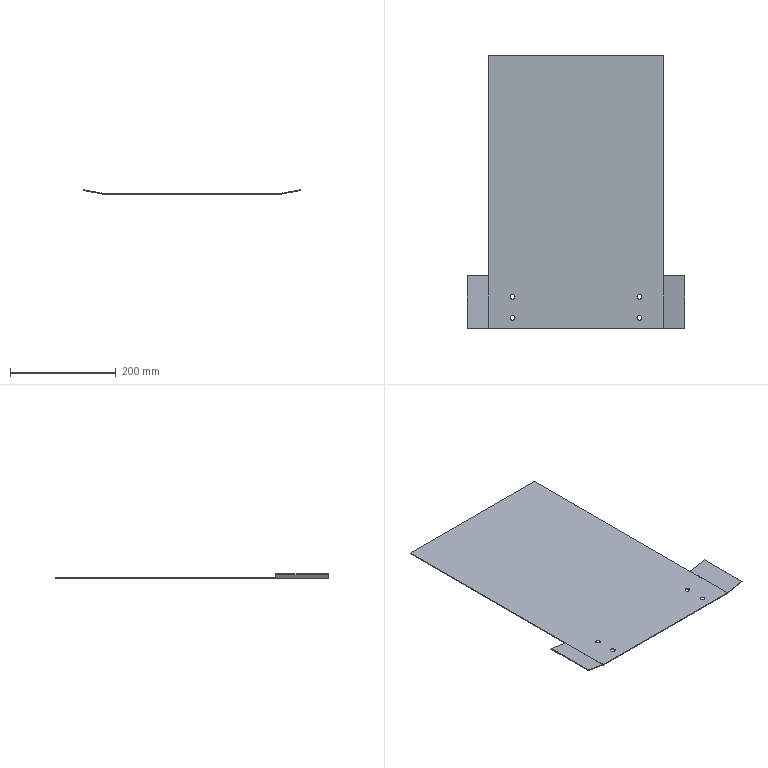Part | SolidWorks | features EdgeFlange 1, FlatPattern 1, ICE 1, SMBaseFlange 1, SheetMetal 1 | 1 solid | 32 faces | box 411.771 x 517 x 8.423 mm | volume 269565 mm3 | plane 20 | cylinder 12 | commonest cylinder face diameters 9 x8 1.473 x2 4.473 x2
STEP:
#1=CARTESIAN_POINT('',(-124.5,-30.,-1.5));
#2=VERTEX_POINT('',#1);
#3=CARTESIAN_POINT('',(-115.5,-30.,-1.5));
#4=VERTEX_POINT('',#3);
#5=CARTESIAN_POINT('',(-120.,-30.,-1.5));
#6=DIRECTION('',(0.,0.,1.));
#7=DIRECTION('',(1.,0.,0.));
#8=AXIS2_PLACEMENT_3D('',#5,#6,#7);
#9=CIRCLE('',#8,4.5);
#10=EDGE_CURVE('',#2,#4,#9,.T.);
#11=ORIENTED_EDGE('',*,*,#10,.F.);
#12=CARTESIAN_POINT('',(-124.5,-30.,0.));
#13=VERTEX_POINT('',#12);
#14=CARTESIAN_POINT('',(-124.5,-30.,-1.5));
#15=DIRECTION('',(0.,0.,1.));
#16=VECTOR('',#15,1000.);
#17=LINE('',#14,#16);
#18=EDGE_CURVE('',#2,#13,#17,.T.);
#19=ORIENTED_EDGE('',*,*,#18,.T.);
#20=CARTESIAN_POINT('',(-115.5,-30.,0.));
#21=VERTEX_POINT('',#20);
#22=CARTESIAN_POINT('',(-120.,-30.,0.));
#23=DIRECTION('',(0.,0.,1.));
#24=DIRECTION('',(1.,0.,0.));
#25=AXIS2_PLACEMENT_3D('',#22,#23,#24);
#26=CIRCLE('',#25,4.5);
#27=EDGE_CURVE('',#13,#21,#26,.T.);
#28=ORIENTED_EDGE('',*,*,#27,.T.);
#29=CARTESIAN_POINT('',(-115.5,-30.,-1.5));
#30=DIRECTION('',(0.,0.,1.));
#31=VECTOR('',#30,1000.);
#32=LINE('',#29,#31);
#33=EDGE_CURVE('',#4,#21,#32,.T.);
#34=ORIENTED_EDGE('',*,*,#33,.F.);
#35=EDGE_LOOP('',(#11,#19,#28,#34));
#36=FACE_OUTER_BOUND('',#35,.T.);
#37=CARTESIAN_POINT('',(-120.,-30.,-1.5));
#38=DIRECTION('',(0.,0.,1.));
#39=DIRECTION('',(1.,0.,0.));
#40=AXIS2_PLACEMENT_3D('',#37,#38,#39);
#41=CYLINDRICAL_SURFACE('',#40,4.5);
#42=ADVANCED_FACE('',(#36),#41,.F.);
#43=CARTESIAN_POINT('',(-124.5,10.,-1.5));
#44=VERTEX_POINT('',#43);
#45=CARTESIAN_POINT('',(-115.5,10.,-1.5));
#46=VERTEX_POINT('',#45);
#47=CARTESIAN_POINT('',(-120.,10.,-1.5));
#48=DIRECTION('',(0.,0.,1.));
#49=DIRECTION('',(1.,0.,0.));
#50=AXIS2_PLACEMENT_3D('',#47,#48,#49);
#51=CIRCLE('',#50,4.5);
#52=EDGE_CURVE('',#44,#46,#51,.T.);
#53=ORIENTED_EDGE('',*,*,#52,.F.);
#54=CARTESIAN_POINT('',(-124.5,10.,0.));
#55=VERTEX_POINT('',#54);
#56=CARTESIAN_POINT('',(-124.5,10.,-1.5));
#57=DIRECTION('',(0.,0.,1.));
#58=VECTOR('',#57,1000.);
#59=LINE('',#56,#58);
#60=EDGE_CURVE('',#44,#55,#59,.T.);
#61=ORIENTED_EDGE('',*,*,#60,.T.);
#62=CARTESIAN_POINT('',(-115.5,10.,0.));
#63=VERTEX_POINT('',#62);
#64=CARTESIAN_POINT('',(-120.,10.,0.));
#65=DIRECTION('',(0.,0.,1.));
#66=DIRECTION('',(1.,0.,0.));
#67=AXIS2_PLACEMENT_3D('',#64,#65,#66);
#68=CIRCLE('',#67,4.5);
#69=EDGE_CURVE('',#55,#63,#68,.T.);
#70=ORIENTED_EDGE('',*,*,#69,.T.);
#71=CARTESIAN_POINT('',(-115.5,10.,-1.5));
#72=DIRECTION('',(0.,0.,1.));
#73=VECTOR('',#72,1000.);
#74=LINE('',#71,#73);
#75=EDGE_CURVE('',#46,#63,#74,.T.);
#76=ORIENTED_EDGE('',*,*,#75,.F.);
#77=EDGE_LOOP('',(#53,#61,#70,#76));
#78=FACE_OUTER_BOUND('',#77,.T.);
#79=CARTESIAN_POINT('',(-120.,10.,-1.5));
#80=DIRECTION('',(0.,0.,1.));
#81=DIRECTION('',(1.,0.,0.));
#82=AXIS2_PLACEMENT_3D('',#79,#80,#81);
#83=CYLINDRICAL_SURFACE('',#82,4.5);
#84=ADVANCED_FACE('',(#78),#83,.F.);
#85=CARTESIAN_POINT('',(115.5,-30.,-1.5));
#86=VERTEX_POINT('',#85);
#87=CARTESIAN_POINT('',(124.5,-30.,-1.5));
#88=VERTEX_POINT('',#87);
#89=CARTESIAN_POINT('',(120.,-30.,-1.5));
#90=DIRECTION('',(0.,0.,1.));
#91=DIRECTION('',(1.,0.,0.));
#92=AXIS2_PLACEMENT_3D('',#89,#90,#91);
#93=CIRCLE('',#92,4.5);
#94=EDGE_CURVE('',#86,#88,#93,.T.);
#95=ORIENTED_EDGE('',*,*,#94,.F.);
#96=CARTESIAN_POINT('',(115.5,-30.,0.));
#97=VERTEX_POINT('',#96);
#98=CARTESIAN_POINT('',(115.5,-30.,-1.5));
#99=DIRECTION('',(0.,0.,1.));
#100=VECTOR('',#99,1000.);
#101=LINE('',#98,#100);
#102=EDGE_CURVE('',#86,#97,#101,.T.);
#103=ORIENTED_EDGE('',*,*,#102,.T.);
#104=CARTESIAN_POINT('',(124.5,-30.,0.));
#105=VERTEX_POINT('',#104);
#106=CARTESIAN_POINT('',(120.,-30.,0.));
#107=DIRECTION('',(0.,0.,1.));
#108=DIRECTION('',(1.,0.,0.));
#109=AXIS2_PLACEMENT_3D('',#106,#107,#108);
#110=CIRCLE('',#109,4.5);
#111=EDGE_CURVE('',#97,#105,#110,.T.);
#112=ORIENTED_EDGE('',*,*,#111,.T.);
#113=CARTESIAN_POINT('',(124.5,-30.,-1.5));
#114=DIRECTION('',(0.,0.,1.));
#115=VECTOR('',#114,1000.);
#116=LINE('',#113,#115);
#117=EDGE_CURVE('',#88,#105,#116,.T.);
#118=ORIENTED_EDGE('',*,*,#117,.F.);
#119=EDGE_LOOP('',(#95,#103,#112,#118));
#120=FACE_OUTER_BOUND('',#119,.T.);
#121=CARTESIAN_POINT('',(120.,-30.,-1.5));
#122=DIRECTION('',(0.,0.,1.));
#123=DIRECTION('',(1.,0.,0.));
#124=AXIS2_PLACEMENT_3D('',#121,#122,#123);
#125=CYLINDRICAL_SURFACE('',#124,4.5);
#126=ADVANCED_FACE('',(#120),#125,.F.);
#127=CARTESIAN_POINT('',(115.5,10.,-1.5));
#128=VERTEX_POINT('',#127);
#129=CARTESIAN_POINT('',(124.5,10.,-1.5));
#130=VERTEX_POINT('',#129);
#131=CARTESIAN_POINT('',(120.,10.,-1.5));
#132=DIRECTION('',(0.,0.,1.));
#133=DIRECTION('',(1.,0.,0.));
#134=AXIS2_PLACEMENT_3D('',#131,#132,#133);
#135=CIRCLE('',#134,4.5);
#136=EDGE_CURVE('',#128,#130,#135,.T.);
#137=ORIENTED_EDGE('',*,*,#136,.F.);
#138=CARTESIAN_POINT('',(115.5,10.,0.));
#139=VERTEX_POINT('',#138);
#140=CARTESIAN_POINT('',(115.5,10.,-1.5));
#141=DIRECTION('',(0.,0.,1.));
#142=VECTOR('',#141,1000.);
#143=LINE('',#140,#142);
#144=EDGE_CURVE('',#128,#139,#143,.T.);
#145=ORIENTED_EDGE('',*,*,#144,.T.);
#146=CARTESIAN_POINT('',(124.5,10.,0.));
#147=VERTEX_POINT('',#146);
#148=CARTESIAN_POINT('',(120.,10.,0.));
#149=DIRECTION('',(0.,0.,1.));
#150=DIRECTION('',(1.,0.,0.));
#151=AXIS2_PLACEMENT_3D('',#148,#149,#150);
#152=CIRCLE('',#151,4.5);
#153=EDGE_CURVE('',#139,#147,#152,.T.);
#154=ORIENTED_EDGE('',*,*,#153,.T.);
#155=CARTESIAN_POINT('',(124.5,10.,-1.5));
#156=DIRECTION('',(0.,0.,1.));
#157=VECTOR('',#156,1000.);
#158=LINE('',#155,#157);
#159=EDGE_CURVE('',#130,#147,#158,.T.);
#160=ORIENTED_EDGE('',*,*,#159,.F.);
#161=EDGE_LOOP('',(#137,#145,#154,#160));
#162=FACE_OUTER_BOUND('',#161,.T.);
#163=CARTESIAN_POINT('',(120.,10.,-1.5));
#164=DIRECTION('',(0.,0.,1.));
#165=DIRECTION('',(1.,0.,0.));
#166=AXIS2_PLACEMENT_3D('',#163,#164,#165);
#167=CYLINDRICAL_SURFACE('',#166,4.5);
#168=ADVANCED_FACE('',(#162),#167,.F.);
#169=CARTESIAN_POINT('',(-120.,-30.,-1.5));
#170=DIRECTION('',(0.,0.,1.));
#171=DIRECTION('',(1.,0.,0.));
#172=AXIS2_PLACEMENT_3D('',#169,#170,#171);
#173=CIRCLE('',#172,4.5);
#174=EDGE_CURVE('',#4,#2,#173,.T.);
#175=ORIENTED_EDGE('',*,*,#174,.T.);
#176=ORIENTED_EDGE('',*,*,#10,.T.);
#177=EDGE_LOOP('',(#175,#176));
#178=FACE_BOUND('',#177,.T.);
#179=CARTESIAN_POINT('',(-120.,10.,-1.5));
#180=DIRECTION('',(0.,0.,1.));
#181=DIRECTION('',(1.,0.,0.));
#182=AXIS2_PLACEMENT_3D('',#179,#180,#181);
#183=CIRCLE('',#182,4.5);
#184=EDGE_CURVE('',#46,#44,#183,.T.);
#185=ORIENTED_EDGE('',*,*,#184,.T.);
#186=ORIENTED_EDGE('',*,*,#52,.T.);
#187=EDGE_LOOP('',(#185,#186));
#188=FACE_BOUND('',#187,.T.);
#189=CARTESIAN_POINT('',(120.,-30.,-1.5));
#190=DIRECTION('',(0.,0.,1.));
#191=DIRECTION('',(1.,0.,0.));
#192=AXIS2_PLACEMENT_3D('',#189,#190,#191);
#193=CIRCLE('',#192,4.5);
#194=EDGE_CURVE('',#88,#86,#193,.T.);
#195=ORIENTED_EDGE('',*,*,#194,.T.);
#196=ORIENTED_EDGE('',*,*,#94,.T.);
#197=EDGE_LOOP('',(#195,#196));
#198=FACE_BOUND('',#197,.T.);
#199=CARTESIAN_POINT('',(120.,10.,-1.5));
#200=DIRECTION('',(0.,0.,1.));
#201=DIRECTION('',(1.,0.,0.));
#202=AXIS2_PLACEMENT_3D('',#199,#200,#201);
#203=CIRCLE('',#202,4.5);
#204=EDGE_CURVE('',#130,#128,#203,.T.);
#205=ORIENTED_EDGE('',*,*,#204,.T.);
#206=ORIENTED_EDGE('',*,*,#136,.T.);
#207=EDGE_LOOP('',(#205,#206));
#208=FACE_BOUND('',#207,.T.);
#209=CARTESIAN_POINT('',(-166.297,-50.,-1.5));
#210=VERTEX_POINT('',#209);
#211=CARTESIAN_POINT('',(-166.297,50.,-1.5));
#212=VERTEX_POINT('',#211);
#213=CARTESIAN_POINT('',(-166.297,-50.,-1.5));
#214=DIRECTION('',(0.,1.,0.));
#215=VECTOR('',#214,1000.);
#216=LINE('',#213,#215);
#217=EDGE_CURVE('',#210,#212,#216,.T.);
#218=ORIENTED_EDGE('',*,*,#217,.T.);
#219=CARTESIAN_POINT('',(-166.297,467.,-1.5));
#220=VERTEX_POINT('',#219);
#221=CARTESIAN_POINT('',(-166.297,467.,-1.5));
#222=DIRECTION('',(0.,-1.,0.));
#223=VECTOR('',#222,1000.);
#224=LINE('',#221,#223);
#225=EDGE_CURVE('',#220,#212,#224,.T.);
#226=ORIENTED_EDGE('',*,*,#225,.F.);
#227=CARTESIAN_POINT('',(166.297,467.,-1.5));
#228=VERTEX_POINT('',#227);
#229=CARTESIAN_POINT('',(166.297,467.,-1.5));
#230=DIRECTION('',(-1.,0.,0.));
#231=VECTOR('',#230,1000.);
#232=LINE('',#229,#231);
#233=EDGE_CURVE('',#228,#220,#232,.T.);
#234=ORIENTED_EDGE('',*,*,#233,.F.);
#235=CARTESIAN_POINT('',(166.297,50.,-1.5));
#236=VERTEX_POINT('',#235);
#237=CARTESIAN_POINT('',(166.297,467.,-1.5));
#238=DIRECTION('',(0.,-1.,0.));
#239=VECTOR('',#238,1000.);
#240=LINE('',#237,#239);
#241=EDGE_CURVE('',#228,#236,#240,.T.);
#242=ORIENTED_EDGE('',*,*,#241,.T.);
#243=CARTESIAN_POINT('',(166.297,-50.,-1.5));
#244=VERTEX_POINT('',#243);
#245=CARTESIAN_POINT('',(166.297,50.,-1.5));
#246=DIRECTION('',(0.,-1.,0.));
#247=VECTOR('',#246,1000.);
#248=LINE('',#245,#247);
#249=EDGE_CURVE('',#236,#244,#248,.T.);
#250=ORIENTED_EDGE('',*,*,#249,.T.);
#251=CARTESIAN_POINT('',(-175.,-50.,-1.5));
#252=DIRECTION('',(1.,0.,0.));
#253=VECTOR('',#252,1000.);
#254=LINE('',#251,#253);
#255=EDGE_CURVE('',#210,#244,#254,.T.);
#256=ORIENTED_EDGE('',*,*,#255,.F.);
#257=EDGE_LOOP('',(#218,#226,#234,#242,#250,#256));
#258=FACE_OUTER_BOUND('',#257,.T.);
#259=CARTESIAN_POINT('',(0.,0.,-1.5));
#260=DIRECTION('',(0.,0.,-1.));
#261=DIRECTION('',(-1.,0.,0.));
#262=AXIS2_PLACEMENT_3D('',#259,#260,#261);
#263=PLANE('',#262);
#264=ADVANCED_FACE('',(#178,#188,#198,#208,#258),#263,.T.);
#265=CARTESIAN_POINT('',(-120.,-30.,0.));
#266=DIRECTION('',(0.,0.,1.));
#267=DIRECTION('',(1.,0.,0.));
#268=AXIS2_PLACEMENT_3D('',#265,#266,#267);
#269=CIRCLE('',#268,4.5);
#270=EDGE_CURVE('',#21,#13,#269,.T.);
#271=ORIENTED_EDGE('',*,*,#270,.F.);
#272=ORIENTED_EDGE('',*,*,#27,.F.);
#273=EDGE_LOOP('',(#271,#272));
#274=FACE_BOUND('',#273,.T.);
#275=CARTESIAN_POINT('',(-120.,10.,0.));
#276=DIRECTION('',(0.,0.,1.));
#277=DIRECTION('',(1.,0.,0.));
#278=AXIS2_PLACEMENT_3D('',#275,#276,#277);
#279=CIRCLE('',#278,4.5);
#280=EDGE_CURVE('',#63,#55,#279,.T.);
#281=ORIENTED_EDGE('',*,*,#280,.F.);
#282=ORIENTED_EDGE('',*,*,#69,.F.);
#283=EDGE_LOOP('',(#281,#282));
#284=FACE_BOUND('',#283,.T.);
#285=CARTESIAN_POINT('',(120.,-30.,0.));
#286=DIRECTION('',(0.,0.,1.));
#287=DIRECTION('',(1.,0.,0.));
#288=AXIS2_PLACEMENT_3D('',#285,#286,#287);
#289=CIRCLE('',#288,4.5);
#290=EDGE_CURVE('',#105,#97,#289,.T.);
#291=ORIENTED_EDGE('',*,*,#290,.F.);
#292=ORIENTED_EDGE('',*,*,#111,.F.);
#293=EDGE_LOOP('',(#291,#292));
#294=FACE_BOUND('',#293,.T.);
#295=CARTESIAN_POINT('',(120.,10.,0.));
#296=DIRECTION('',(0.,0.,1.));
#297=DIRECTION('',(1.,0.,0.));
#298=AXIS2_PLACEMENT_3D('',#295,#296,#297);
#299=CIRCLE('',#298,4.5);
#300=EDGE_CURVE('',#147,#139,#299,.T.);
#301=ORIENTED_EDGE('',*,*,#300,.F.);
#302=ORIENTED_EDGE('',*,*,#153,.F.);
#303=EDGE_LOOP('',(#301,#302));
#304=FACE_BOUND('',#303,.T.);
#305=CARTESIAN_POINT('',(166.297,50.,0.));
#306=VERTEX_POINT('',#305);
#307=CARTESIAN_POINT('',(166.297,-50.,0.));
#308=VERTEX_POINT('',#307);
#309=CARTESIAN_POINT('',(166.297,50.,0.));
#310=DIRECTION('',(0.,-1.,0.));
#311=VECTOR('',#310,1000.);
#312=LINE('',#309,#311);
#313=EDGE_CURVE('',#306,#308,#312,.T.);
#314=ORIENTED_EDGE('',*,*,#313,.F.);
#315=CARTESIAN_POINT('',(166.297,467.,0.));
#316=VERTEX_POINT('',#315);
#317=CARTESIAN_POINT('',(166.297,467.,0.));
#318=DIRECTION('',(0.,-1.,0.));
#319=VECTOR('',#318,1000.);
#320=LINE('',#317,#319);
#321=EDGE_CURVE('',#316,#306,#320,.T.);
#322=ORIENTED_EDGE('',*,*,#321,.F.);
#323=CARTESIAN_POINT('',(-166.297,467.,0.));
#324=VERTEX_POINT('',#323);
#325=CARTESIAN_POINT('',(-166.297,467.,0.));
#326=DIRECTION('',(1.,0.,0.));
#327=VECTOR('',#326,1000.);
#328=LINE('',#325,#327);
#329=EDGE_CURVE('',#324,#316,#328,.T.);
#330=ORIENTED_EDGE('',*,*,#329,.F.);
#331=CARTESIAN_POINT('',(-166.297,50.,0.));
#332=VERTEX_POINT('',#331);
#333=CARTESIAN_POINT('',(-166.297,467.,0.));
#334=DIRECTION('',(0.,-1.,0.));
#335=VECTOR('',#334,1000.);
#336=LINE('',#333,#335);
#337=EDGE_CURVE('',#324,#332,#336,.T.);
#338=ORIENTED_EDGE('',*,*,#337,.T.);
#339=CARTESIAN_POINT('',(-166.297,-50.,0.));
#340=VERTEX_POINT('',#339);
#341=CARTESIAN_POINT('',(-166.297,-50.,0.));
#342=DIRECTION('',(0.,1.,0.));
#343=VECTOR('',#342,1000.);
#344=LINE('',#341,#343);
#345=EDGE_CURVE('',#340,#332,#344,.T.);
#346=ORIENTED_EDGE('',*,*,#345,.F.);
#347=CARTESIAN_POINT('',(-175.,-50.,0.));
#348=DIRECTION('',(1.,0.,0.));
#349=VECTOR('',#348,1000.);
#350=LINE('',#347,#349);
#351=EDGE_CURVE('',#340,#308,#350,.T.);
#352=ORIENTED_EDGE('',*,*,#351,.T.);
#353=EDGE_LOOP('',(#314,#322,#330,#338,#346,#352));
#354=FACE_OUTER_BOUND('',#353,.T.);
#355=CARTESIAN_POINT('',(0.,0.,0.));
#356=DIRECTION('',(0.,0.,-1.));
#357=DIRECTION('',(-1.,0.,0.));
#358=AXIS2_PLACEMENT_3D('',#355,#356,#357);
#359=PLANE('',#358);
#360=ADVANCED_FACE('',(#274,#284,#294,#304,#354),#359,.F.);
#361=CARTESIAN_POINT('',(166.297,-50.,0.));
#362=DIRECTION('',(0.,0.,-1.));
#363=VECTOR('',#362,1000.);
#364=LINE('',#361,#363);
#365=EDGE_CURVE('',#308,#244,#364,.T.);
#366=ORIENTED_EDGE('',*,*,#365,.F.);
#367=ORIENTED_EDGE('',*,*,#351,.F.);
#368=CARTESIAN_POINT('',(-166.297,-50.,0.));
#369=DIRECTION('',(0.,0.,-1.));
#370=VECTOR('',#369,1000.);
#371=LINE('',#368,#370);
#372=EDGE_CURVE('',#340,#210,#371,.T.);
#373=ORIENTED_EDGE('',*,*,#372,.T.);
#374=ORIENTED_EDGE('',*,*,#255,.T.);
#375=EDGE_LOOP('',(#366,#367,#373,#374));
#376=FACE_OUTER_BOUND('',#375,.T.);
#377=CARTESIAN_POINT('',(-175.,-50.,-1.5));
#378=DIRECTION('',(0.,-1.,0.));
#379=DIRECTION('',(0.,0.,-1.));
#380=AXIS2_PLACEMENT_3D('',#377,#378,#379);
#381=PLANE('',#380);
#382=ADVANCED_FACE('',(#376),#381,.T.);
#383=ORIENTED_EDGE('',*,*,#144,.F.);
#384=ORIENTED_EDGE('',*,*,#204,.F.);
#385=ORIENTED_EDGE('',*,*,#159,.T.);
#386=ORIENTED_EDGE('',*,*,#300,.T.);
#387=EDGE_LOOP('',(#383,#384,#385,#386));
#388=FACE_OUTER_BOUND('',#387,.T.);
#389=CARTESIAN_POINT('',(120.,10.,-1.5));
#390=DIRECTION('',(0.,0.,1.));
#391=DIRECTION('',(1.,0.,0.));
#392=AXIS2_PLACEMENT_3D('',#389,#390,#391);
#393=CYLINDRICAL_SURFACE('',#392,4.5);
#394=ADVANCED_FACE('',(#388),#393,.F.);
#395=ORIENTED_EDGE('',*,*,#102,.F.);
#396=ORIENTED_EDGE('',*,*,#194,.F.);
#397=ORIENTED_EDGE('',*,*,#117,.T.);
#398=ORIENTED_EDGE('',*,*,#290,.T.);
#399=EDGE_LOOP('',(#395,#396,#397,#398));
#400=FACE_OUTER_BOUND('',#399,.T.);
#401=CARTESIAN_POINT('',(120.,-30.,-1.5));
#402=DIRECTION('',(0.,0.,1.));
#403=DIRECTION('',(1.,0.,0.));
#404=AXIS2_PLACEMENT_3D('',#401,#402,#403);
#405=CYLINDRICAL_SURFACE('',#404,4.5);
#406=ADVANCED_FACE('',(#400),#405,.F.);
#407=ORIENTED_EDGE('',*,*,#60,.F.);
#408=ORIENTED_EDGE('',*,*,#184,.F.);
#409=ORIENTED_EDGE('',*,*,#75,.T.);
#410=ORIENTED_EDGE('',*,*,#280,.T.);
#411=EDGE_LOOP('',(#407,#408,#409,#410));
#412=FACE_OUTER_BOUND('',#411,.T.);
#413=CARTESIAN_POINT('',(-120.,10.,-1.5));
#414=DIRECTION('',(0.,0.,1.));
#415=DIRECTION('',(1.,0.,0.));
#416=AXIS2_PLACEMENT_3D('',#413,#414,#415);
#417=CYLINDRICAL_SURFACE('',#416,4.5);
#418=ADVANCED_FACE('',(#412),#417,.F.);
#419=ORIENTED_EDGE('',*,*,#18,.F.);
#420=ORIENTED_EDGE('',*,*,#174,.F.);
#421=ORIENTED_EDGE('',*,*,#33,.T.);
#422=ORIENTED_EDGE('',*,*,#270,.T.);
#423=EDGE_LOOP('',(#419,#420,#421,#422));
#424=FACE_OUTER_BOUND('',#423,.T.);
#425=CARTESIAN_POINT('',(-120.,-30.,-1.5));
#426=DIRECTION('',(0.,0.,1.));
#427=DIRECTION('',(1.,0.,0.));
#428=AXIS2_PLACEMENT_3D('',#425,#426,#427);
#429=CYLINDRICAL_SURFACE('',#428,4.5);
#430=ADVANCED_FACE('',(#424),#429,.F.);
#431=CARTESIAN_POINT('',(-166.425,50.,0.01119));
#432=VERTEX_POINT('',#431);
#433=CARTESIAN_POINT('',(-166.686,50.,-1.466));
#434=VERTEX_POINT('',#433);
#435=CARTESIAN_POINT('',(-166.686,50.,-1.466));
#436=DIRECTION('',(-0.1736,0.,-0.9848));
#437=VECTOR('',#436,1000.);
#438=LINE('',#435,#437);
#439=EDGE_CURVE('',#432,#434,#438,.T.);
#440=ORIENTED_EDGE('',*,*,#439,.F.);
#441=CARTESIAN_POINT('',(-166.297,50.,0.7366));
#442=DIRECTION('',(0.,1.,0.));
#443=DIRECTION('',(0.,0.,-1.));
#444=AXIS2_PLACEMENT_3D('',#441,#442,#443);
#445=CIRCLE('',#444,0.7366);
#446=EDGE_CURVE('',#332,#432,#445,.T.);
#447=ORIENTED_EDGE('',*,*,#446,.F.);
#448=CARTESIAN_POINT('',(-166.297,50.,0.));
#449=DIRECTION('',(0.,0.,-1.));
#450=VECTOR('',#449,1000.);
#451=LINE('',#448,#450);
#452=EDGE_CURVE('',#332,#212,#451,.T.);
#453=ORIENTED_EDGE('',*,*,#452,.T.);
#454=CARTESIAN_POINT('',(-166.297,50.,0.7366));
#455=DIRECTION('',(0.,1.,0.));
#456=DIRECTION('',(0.,0.,-1.));
#457=AXIS2_PLACEMENT_3D('',#454,#455,#456);
#458=CIRCLE('',#457,2.237);
#459=EDGE_CURVE('',#212,#434,#458,.T.);
#460=ORIENTED_EDGE('',*,*,#459,.T.);
#461=EDGE_LOOP('',(#440,#447,#453,#460));
#462=FACE_OUTER_BOUND('',#461,.T.);
#463=CARTESIAN_POINT('',(-166.297,50.,0.7366));
#464=DIRECTION('',(0.,1.,0.));
#465=DIRECTION('',(0.,0.,1.));
#466=AXIS2_PLACEMENT_3D('',#463,#464,#465);
#467=PLANE('',#466);
#468=ADVANCED_FACE('',(#462),#467,.T.);
#469=CARTESIAN_POINT('',(-166.425,-50.,0.01119));
#470=VERTEX_POINT('',#469);
#471=CARTESIAN_POINT('',(-166.297,-50.,0.7366));
#472=DIRECTION('',(0.,-1.,0.));
#473=DIRECTION('',(0.,0.,-1.));
#474=AXIS2_PLACEMENT_3D('',#471,#472,#473);
#475=CIRCLE('',#474,0.7366);
#476=EDGE_CURVE('',#470,#340,#475,.T.);
#477=ORIENTED_EDGE('',*,*,#476,.F.);
#478=CARTESIAN_POINT('',(-166.686,-50.,-1.466));
#479=VERTEX_POINT('',#478);
#480=CARTESIAN_POINT('',(-166.425,-50.,0.01119));
#481=DIRECTION('',(-0.1736,0.,-0.9848));
#482=VECTOR('',#481,1000.);
#483=LINE('',#480,#482);
#484=EDGE_CURVE('',#470,#479,#483,.T.);
#485=ORIENTED_EDGE('',*,*,#484,.T.);
#486=CARTESIAN_POINT('',(-166.297,-50.,0.7366));
#487=DIRECTION('',(0.,-1.,0.));
#488=DIRECTION('',(0.,0.,-1.));
#489=AXIS2_PLACEMENT_3D('',#486,#487,#488);
#490=CIRCLE('',#489,2.237);
#491=EDGE_CURVE('',#479,#210,#490,.T.);
#492=ORIENTED_EDGE('',*,*,#491,.T.);
#493=ORIENTED_EDGE('',*,*,#372,.F.);
#494=EDGE_LOOP('',(#477,#485,#492,#493));
#495=FACE_OUTER_BOUND('',#494,.T.);
#496=CARTESIAN_POINT('',(-166.297,-50.,0.7366));
#497=DIRECTION('',(0.,1.,0.));
#498=DIRECTION('',(0.,0.,1.));
#499=AXIS2_PLACEMENT_3D('',#496,#497,#498);
#500=PLANE('',#499);
#501=ADVANCED_FACE('',(#495),#500,.F.);
#502=ORIENTED_EDGE('',*,*,#217,.F.);
#503=ORIENTED_EDGE('',*,*,#491,.F.);
#504=CARTESIAN_POINT('',(-166.686,50.,-1.466));
#505=DIRECTION('',(0.,1.,0.));
#506=VECTOR('',#505,1000.);
#507=LINE('',#504,#506);
#508=EDGE_CURVE('',#479,#434,#507,.T.);
#509=ORIENTED_EDGE('',*,*,#508,.T.);
#510=ORIENTED_EDGE('',*,*,#459,.F.);
#511=EDGE_LOOP('',(#502,#503,#509,#510));
#512=FACE_OUTER_BOUND('',#511,.T.);
#513=CARTESIAN_POINT('',(-166.297,-50.,0.7366));
#514=DIRECTION('',(0.,-1.,0.));
#515=DIRECTION('',(-0.1736,0.,-0.9848));
#516=AXIS2_PLACEMENT_3D('',#513,#514,#515);
#517=CYLINDRICAL_SURFACE('',#516,2.237);
#518=ADVANCED_FACE('',(#512),#517,.T.);
#519=ORIENTED_EDGE('',*,*,#345,.T.);
#520=ORIENTED_EDGE('',*,*,#446,.T.);
#521=CARTESIAN_POINT('',(-166.425,50.,0.01119));
#522=DIRECTION('',(0.,-1.,0.));
#523=VECTOR('',#522,1000.);
#524=LINE('',#521,#523);
#525=EDGE_CURVE('',#432,#470,#524,.T.);
#526=ORIENTED_EDGE('',*,*,#525,.T.);
#527=ORIENTED_EDGE('',*,*,#476,.T.);
#528=EDGE_LOOP('',(#519,#520,#526,#527));
#529=FACE_OUTER_BOUND('',#528,.T.);
#530=CARTESIAN_POINT('',(-166.297,-50.,0.7366));
#531=DIRECTION('',(0.,-1.,0.));
#532=DIRECTION('',(-0.1736,0.,-0.9848));
#533=AXIS2_PLACEMENT_3D('',#530,#531,#532);
#534=CYLINDRICAL_SURFACE('',#533,0.7366);
#535=ADVANCED_FACE('',(#529),#534,.F.);
#536=ORIENTED_EDGE('',*,*,#439,.T.);
#537=CARTESIAN_POINT('',(-205.885,50.,5.446));
#538=VERTEX_POINT('',#537);
#539=CARTESIAN_POINT('',(3.101,50.,-31.404));
#540=DIRECTION('',(0.9848,0.,-0.1736));
#541=VECTOR('',#540,1000.);
#542=LINE('',#539,#541);
#543=EDGE_CURVE('',#538,#434,#542,.T.);
#544=ORIENTED_EDGE('',*,*,#543,.F.);
#545=CARTESIAN_POINT('',(-205.625,50.,6.923));
#546=VERTEX_POINT('',#545);
#547=CARTESIAN_POINT('',(-205.885,50.,5.446));
#548=DIRECTION('',(0.1736,0.,0.9848));
#549=VECTOR('',#548,1000.);
#550=LINE('',#547,#549);
#551=EDGE_CURVE('',#538,#546,#550,.T.);
#552=ORIENTED_EDGE('',*,*,#551,.T.);
#553=CARTESIAN_POINT('',(-166.362,50.,0.));
#554=DIRECTION('',(0.9848,0.,-0.1736));
#555=VECTOR('',#554,1000.);
#556=LINE('',#553,#555);
#557=EDGE_CURVE('',#546,#432,#556,.T.);
#558=ORIENTED_EDGE('',*,*,#557,.T.);
#559=EDGE_LOOP('',(#536,#544,#552,#558));
#560=FACE_OUTER_BOUND('',#559,.T.);
#561=CARTESIAN_POINT('',(-166.622,50.,-1.477));
#562=DIRECTION('',(0.,-1.,0.));
#563=DIRECTION('',(1.,0.,0.));
#564=AXIS2_PLACEMENT_3D('',#561,#562,#563);
#565=PLANE('',#564);
#566=ADVANCED_FACE('',(#560),#565,.F.);
#567=ORIENTED_EDGE('',*,*,#484,.F.);
#568=CARTESIAN_POINT('',(-205.625,-50.,6.923));
#569=VERTEX_POINT('',#568);
#570=CARTESIAN_POINT('',(-205.625,-50.,6.923));
#571=DIRECTION('',(-0.9848,0.,0.1736));
#572=VECTOR('',#571,1000.);
#573=LINE('',#570,#572);
#574=EDGE_CURVE('',#470,#569,#573,.T.);
#575=ORIENTED_EDGE('',*,*,#574,.T.);
#576=CARTESIAN_POINT('',(-205.885,-50.,5.446));
#577=VERTEX_POINT('',#576);
#578=CARTESIAN_POINT('',(-205.885,-50.,5.446));
#579=DIRECTION('',(0.1736,0.,0.9848));
#580=VECTOR('',#579,1000.);
#581=LINE('',#578,#580);
#582=EDGE_CURVE('',#577,#569,#581,.T.);
#583=ORIENTED_EDGE('',*,*,#582,.F.);
#584=CARTESIAN_POINT('',(3.101,-50.,-31.404));
#585=DIRECTION('',(-0.9848,0.,0.1736));
#586=VECTOR('',#585,1000.);
#587=LINE('',#584,#586);
#588=EDGE_CURVE('',#479,#577,#587,.T.);
#589=ORIENTED_EDGE('',*,*,#588,.F.);
#590=EDGE_LOOP('',(#567,#575,#583,#589));
#591=FACE_OUTER_BOUND('',#590,.T.);
#592=CARTESIAN_POINT('',(-205.885,-50.,5.446));
#593=DIRECTION('',(0.,1.,0.));
#594=DIRECTION('',(-1.,0.,0.));
#595=AXIS2_PLACEMENT_3D('',#592,#593,#594);
#596=PLANE('',#595);
#597=ADVANCED_FACE('',(#591),#596,.F.);
#598=ORIENTED_EDGE('',*,*,#508,.F.);
#599=ORIENTED_EDGE('',*,*,#588,.T.);
#600=CARTESIAN_POINT('',(-205.885,0.,5.446));
#601=DIRECTION('',(0.,1.,0.));
#602=VECTOR('',#601,1000.);
#603=LINE('',#600,#602);
#604=EDGE_CURVE('',#577,#538,#603,.T.);
#605=ORIENTED_EDGE('',*,*,#604,.T.);
#606=ORIENTED_EDGE('',*,*,#543,.T.);
#607=EDGE_LOOP('',(#598,#599,#605,#606));
#608=FACE_OUTER_BOUND('',#607,.T.);
#609=CARTESIAN_POINT('',(3.101,0.,-31.404));
#610=DIRECTION('',(0.1736,0.,0.9848));
#611=DIRECTION('',(0.9848,0.,-0.1736));
#612=AXIS2_PLACEMENT_3D('',#609,#610,#611);
#613=PLANE('',#612);
#614=ADVANCED_FACE('',(#608),#613,.F.);
#615=ORIENTED_EDGE('',*,*,#574,.F.);
#616=ORIENTED_EDGE('',*,*,#525,.F.);
#617=ORIENTED_EDGE('',*,*,#557,.F.);
#618=CARTESIAN_POINT('',(-205.625,50.,6.923));
#619=DIRECTION('',(0.,1.,0.));
#620=VECTOR('',#619,1000.);
#621=LINE('',#618,#620);
#622=EDGE_CURVE('',#569,#546,#621,.T.);
#623=ORIENTED_EDGE('',*,*,#622,.F.);
#624=EDGE_LOOP('',(#615,#616,#617,#623));
#625=FACE_OUTER_BOUND('',#624,.T.);
#626=CARTESIAN_POINT('',(3.361,0.,-29.927));
#627=DIRECTION('',(0.1736,0.,0.9848));
#628=DIRECTION('',(0.9848,0.,-0.1736));
#629=AXIS2_PLACEMENT_3D('',#626,#627,#628);
#630=PLANE('',#629);
#631=ADVANCED_FACE('',(#625),#630,.T.);
#632=ORIENTED_EDGE('',*,*,#622,.T.);
#633=ORIENTED_EDGE('',*,*,#551,.F.);
#634=ORIENTED_EDGE('',*,*,#604,.F.);
#635=ORIENTED_EDGE('',*,*,#582,.T.);
#636=EDGE_LOOP('',(#632,#633,#634,#635));
#637=FACE_OUTER_BOUND('',#636,.T.);
#638=CARTESIAN_POINT('',(-205.885,50.,5.446));
#639=DIRECTION('',(0.9848,0.,-0.1736));
#640=DIRECTION('',(-0.1736,0.,-0.9848));
#641=AXIS2_PLACEMENT_3D('',#638,#639,#640);
#642=PLANE('',#641);
#643=ADVANCED_FACE('',(#637),#642,.F.);
#644=CARTESIAN_POINT('',(166.425,-50.,0.01119));
#645=VERTEX_POINT('',#644);
#646=CARTESIAN_POINT('',(166.686,-50.,-1.466));
#647=VERTEX_POINT('',#646);
#648=CARTESIAN_POINT('',(166.686,-50.,-1.466));
#649=DIRECTION('',(0.1736,0.,-0.9848));
#650=VECTOR('',#649,1000.);
#651=LINE('',#648,#650);
#652=EDGE_CURVE('',#645,#647,#651,.T.);
#653=ORIENTED_EDGE('',*,*,#652,.F.);
#654=CARTESIAN_POINT('',(166.297,-50.,0.7366));
#655=DIRECTION('',(0.,-1.,0.));
#656=DIRECTION('',(0.,0.,1.));
#657=AXIS2_PLACEMENT_3D('',#654,#655,#656);
#658=CIRCLE('',#657,0.7366);
#659=EDGE_CURVE('',#308,#645,#658,.T.);
#660=ORIENTED_EDGE('',*,*,#659,.F.);
#661=ORIENTED_EDGE('',*,*,#365,.T.);
#662=CARTESIAN_POINT('',(166.297,-50.,0.7366));
#663=DIRECTION('',(0.,-1.,0.));
#664=DIRECTION('',(0.,0.,1.));
#665=AXIS2_PLACEMENT_3D('',#662,#663,#664);
#666=CIRCLE('',#665,2.237);
#667=EDGE_CURVE('',#244,#647,#666,.T.);
#668=ORIENTED_EDGE('',*,*,#667,.T.);
#669=EDGE_LOOP('',(#653,#660,#661,#668));
#670=FACE_OUTER_BOUND('',#669,.T.);
#671=CARTESIAN_POINT('',(166.297,-50.,0.7366));
#672=DIRECTION('',(0.,-1.,0.));
#673=DIRECTION('',(0.,0.,-1.));
#674=AXIS2_PLACEMENT_3D('',#671,#672,#673);
#675=PLANE('',#674);
#676=ADVANCED_FACE('',(#670),#675,.T.);
#677=CARTESIAN_POINT('',(166.425,50.,0.01119));
#678=VERTEX_POINT('',#677);
#679=CARTESIAN_POINT('',(166.297,50.,0.7366));
#680=DIRECTION('',(0.,1.,0.));
#681=DIRECTION('',(0.,0.,1.));
#682=AXIS2_PLACEMENT_3D('',#679,#680,#681);
#683=CIRCLE('',#682,0.7366);
#684=EDGE_CURVE('',#678,#306,#683,.T.);
#685=ORIENTED_EDGE('',*,*,#684,.F.);
#686=CARTESIAN_POINT('',(166.686,50.,-1.466));
#687=VERTEX_POINT('',#686);
#688=CARTESIAN_POINT('',(166.425,50.,0.01119));
#689=DIRECTION('',(0.1736,0.,-0.9848));
#690=VECTOR('',#689,1000.);
#691=LINE('',#688,#690);
#692=EDGE_CURVE('',#678,#687,#691,.T.);
#693=ORIENTED_EDGE('',*,*,#692,.T.);
#694=CARTESIAN_POINT('',(166.297,50.,0.7366));
#695=DIRECTION('',(0.,1.,0.));
#696=DIRECTION('',(0.,0.,1.));
#697=AXIS2_PLACEMENT_3D('',#694,#695,#696);
#698=CIRCLE('',#697,2.237);
#699=EDGE_CURVE('',#687,#236,#698,.T.);
#700=ORIENTED_EDGE('',*,*,#699,.T.);
#701=CARTESIAN_POINT('',(166.297,50.,0.));
#702=DIRECTION('',(0.,0.,-1.));
#703=VECTOR('',#702,1000.);
#704=LINE('',#701,#703);
#705=EDGE_CURVE('',#306,#236,#704,.T.);
#706=ORIENTED_EDGE('',*,*,#705,.F.);
#707=EDGE_LOOP('',(#685,#693,#700,#706));
#708=FACE_OUTER_BOUND('',#707,.T.);
#709=CARTESIAN_POINT('',(166.297,50.,0.7366));
#710=DIRECTION('',(0.,-1.,0.));
#711=DIRECTION('',(0.,0.,-1.));
#712=AXIS2_PLACEMENT_3D('',#709,#710,#711);
#713=PLANE('',#712);
#714=ADVANCED_FACE('',(#708),#713,.F.);
#715=ORIENTED_EDGE('',*,*,#249,.F.);
#716=ORIENTED_EDGE('',*,*,#699,.F.);
#717=CARTESIAN_POINT('',(166.686,-50.,-1.466));
#718=DIRECTION('',(0.,-1.,0.));
#719=VECTOR('',#718,1000.);
#720=LINE('',#717,#719);
#721=EDGE_CURVE('',#687,#647,#720,.T.);
#722=ORIENTED_EDGE('',*,*,#721,.T.);
#723=ORIENTED_EDGE('',*,*,#667,.F.);
#724=EDGE_LOOP('',(#715,#716,#722,#723));
#725=FACE_OUTER_BOUND('',#724,.T.);
#726=CARTESIAN_POINT('',(166.297,50.,0.7366));
#727=DIRECTION('',(0.,1.,0.));
#728=DIRECTION('',(0.1736,0.,-0.9848));
#729=AXIS2_PLACEMENT_3D('',#726,#727,#728);
#730=CYLINDRICAL_SURFACE('',#729,2.237);
#731=ADVANCED_FACE('',(#725),#730,.T.);
#732=ORIENTED_EDGE('',*,*,#313,.T.);
#733=ORIENTED_EDGE('',*,*,#659,.T.);
#734=CARTESIAN_POINT('',(166.425,-50.,0.01119));
#735=DIRECTION('',(0.,1.,0.));
#736=VECTOR('',#735,1000.);
#737=LINE('',#734,#736);
#738=EDGE_CURVE('',#645,#678,#737,.T.);
#739=ORIENTED_EDGE('',*,*,#738,.T.);
#740=ORIENTED_EDGE('',*,*,#684,.T.);
#741=EDGE_LOOP('',(#732,#733,#739,#740));
#742=FACE_OUTER_BOUND('',#741,.T.);
#743=CARTESIAN_POINT('',(166.297,50.,0.7366));
#744=DIRECTION('',(0.,1.,0.));
#745=DIRECTION('',(0.1736,0.,-0.9848));
#746=AXIS2_PLACEMENT_3D('',#743,#744,#745);
#747=CYLINDRICAL_SURFACE('',#746,0.7366);
#748=ADVANCED_FACE('',(#742),#747,.F.);
#749=ORIENTED_EDGE('',*,*,#652,.T.);
#750=CARTESIAN_POINT('',(205.885,-50.,5.446));
#751=VERTEX_POINT('',#750);
#752=CARTESIAN_POINT('',(-3.101,-50.,-31.404));
#753=DIRECTION('',(-0.9848,0.,-0.1736));
#754=VECTOR('',#753,1000.);
#755=LINE('',#752,#754);
#756=EDGE_CURVE('',#751,#647,#755,.T.);
#757=ORIENTED_EDGE('',*,*,#756,.F.);
#758=CARTESIAN_POINT('',(205.625,-50.,6.923));
#759=VERTEX_POINT('',#758);
#760=CARTESIAN_POINT('',(205.885,-50.,5.446));
#761=DIRECTION('',(-0.1736,0.,0.9848));
#762=VECTOR('',#761,1000.);
#763=LINE('',#760,#762);
#764=EDGE_CURVE('',#751,#759,#763,.T.);
#765=ORIENTED_EDGE('',*,*,#764,.T.);
#766=CARTESIAN_POINT('',(166.362,-50.,0.));
#767=DIRECTION('',(-0.9848,0.,-0.1736));
#768=VECTOR('',#767,1000.);
#769=LINE('',#766,#768);
#770=EDGE_CURVE('',#759,#645,#769,.T.);
#771=ORIENTED_EDGE('',*,*,#770,.T.);
#772=EDGE_LOOP('',(#749,#757,#765,#771));
#773=FACE_OUTER_BOUND('',#772,.T.);
#774=CARTESIAN_POINT('',(166.622,-50.,-1.477));
#775=DIRECTION('',(0.,1.,0.));
#776=DIRECTION('',(-1.,0.,0.));
#777=AXIS2_PLACEMENT_3D('',#774,#775,#776);
#778=PLANE('',#777);
#779=ADVANCED_FACE('',(#773),#778,.F.);
#780=ORIENTED_EDGE('',*,*,#692,.F.);
#781=CARTESIAN_POINT('',(205.625,50.,6.923));
#782=VERTEX_POINT('',#781);
#783=CARTESIAN_POINT('',(205.625,50.,6.923));
#784=DIRECTION('',(0.9848,0.,0.1736));
#785=VECTOR('',#784,1000.);
#786=LINE('',#783,#785);
#787=EDGE_CURVE('',#678,#782,#786,.T.);
#788=ORIENTED_EDGE('',*,*,#787,.T.);
#789=CARTESIAN_POINT('',(205.885,50.,5.446));
#790=VERTEX_POINT('',#789);
#791=CARTESIAN_POINT('',(205.885,50.,5.446));
#792=DIRECTION('',(-0.1736,0.,0.9848));
#793=VECTOR('',#792,1000.);
#794=LINE('',#791,#793);
#795=EDGE_CURVE('',#790,#782,#794,.T.);
#796=ORIENTED_EDGE('',*,*,#795,.F.);
#797=CARTESIAN_POINT('',(-3.101,50.,-31.404));
#798=DIRECTION('',(0.9848,0.,0.1736));
#799=VECTOR('',#798,1000.);
#800=LINE('',#797,#799);
#801=EDGE_CURVE('',#687,#790,#800,.T.);
#802=ORIENTED_EDGE('',*,*,#801,.F.);
#803=EDGE_LOOP('',(#780,#788,#796,#802));
#804=FACE_OUTER_BOUND('',#803,.T.);
#805=CARTESIAN_POINT('',(205.885,50.,5.446));
#806=DIRECTION('',(0.,-1.,0.));
#807=DIRECTION('',(1.,0.,0.));
#808=AXIS2_PLACEMENT_3D('',#805,#806,#807);
#809=PLANE('',#808);
#810=ADVANCED_FACE('',(#804),#809,.F.);
#811=ORIENTED_EDGE('',*,*,#721,.F.);
#812=ORIENTED_EDGE('',*,*,#801,.T.);
#813=CARTESIAN_POINT('',(205.885,0.,5.446));
#814=DIRECTION('',(0.,-1.,0.));
#815=VECTOR('',#814,1000.);
#816=LINE('',#813,#815);
#817=EDGE_CURVE('',#790,#751,#816,.T.);
#818=ORIENTED_EDGE('',*,*,#817,.T.);
#819=ORIENTED_EDGE('',*,*,#756,.T.);
#820=EDGE_LOOP('',(#811,#812,#818,#819));
#821=FACE_OUTER_BOUND('',#820,.T.);
#822=CARTESIAN_POINT('',(-3.101,0.,-31.404));
#823=DIRECTION('',(-0.1736,0.,0.9848));
#824=DIRECTION('',(0.9848,0.,0.1736));
#825=AXIS2_PLACEMENT_3D('',#822,#823,#824);
#826=PLANE('',#825);
#827=ADVANCED_FACE('',(#821),#826,.F.);
#828=ORIENTED_EDGE('',*,*,#787,.F.);
#829=ORIENTED_EDGE('',*,*,#738,.F.);
#830=ORIENTED_EDGE('',*,*,#770,.F.);
#831=CARTESIAN_POINT('',(205.625,-50.,6.923));
#832=DIRECTION('',(0.,-1.,0.));
#833=VECTOR('',#832,1000.);
#834=LINE('',#831,#833);
#835=EDGE_CURVE('',#782,#759,#834,.T.);
#836=ORIENTED_EDGE('',*,*,#835,.F.);
#837=EDGE_LOOP('',(#828,#829,#830,#836));
#838=FACE_OUTER_BOUND('',#837,.T.);
#839=CARTESIAN_POINT('',(-3.361,0.,-29.927));
#840=DIRECTION('',(-0.1736,0.,0.9848));
#841=DIRECTION('',(0.9848,0.,0.1736));
#842=AXIS2_PLACEMENT_3D('',#839,#840,#841);
#843=PLANE('',#842);
#844=ADVANCED_FACE('',(#838),#843,.T.);
#845=ORIENTED_EDGE('',*,*,#835,.T.);
#846=ORIENTED_EDGE('',*,*,#764,.F.);
#847=ORIENTED_EDGE('',*,*,#817,.F.);
#848=ORIENTED_EDGE('',*,*,#795,.T.);
#849=EDGE_LOOP('',(#845,#846,#847,#848));
#850=FACE_OUTER_BOUND('',#849,.T.);
#851=CARTESIAN_POINT('',(205.885,-50.,5.446));
#852=DIRECTION('',(-0.9848,0.,-0.1736));
#853=DIRECTION('',(-0.1736,0.,0.9848));
#854=AXIS2_PLACEMENT_3D('',#851,#852,#853);
#855=PLANE('',#854);
#856=ADVANCED_FACE('',(#850),#855,.F.);
#857=ORIENTED_EDGE('',*,*,#452,.F.);
#858=ORIENTED_EDGE('',*,*,#337,.F.);
#859=CARTESIAN_POINT('',(-166.297,467.,-1.5));
#860=DIRECTION('',(0.,0.,1.));
#861=VECTOR('',#860,1000.);
#862=LINE('',#859,#861);
#863=EDGE_CURVE('',#220,#324,#862,.T.);
#864=ORIENTED_EDGE('',*,*,#863,.F.);
#865=ORIENTED_EDGE('',*,*,#225,.T.);
#866=EDGE_LOOP('',(#857,#858,#864,#865));
#867=FACE_OUTER_BOUND('',#866,.T.);
#868=CARTESIAN_POINT('',(-166.297,467.,-1.5));
#869=DIRECTION('',(1.,0.,0.));
#870=DIRECTION('',(0.,0.,-1.));
#871=AXIS2_PLACEMENT_3D('',#868,#869,#870);
#872=PLANE('',#871);
#873=ADVANCED_FACE('',(#867),#872,.F.);
#874=ORIENTED_EDGE('',*,*,#705,.T.);
#875=ORIENTED_EDGE('',*,*,#241,.F.);
#876=CARTESIAN_POINT('',(166.297,467.,0.));
#877=DIRECTION('',(0.,0.,-1.));
#878=VECTOR('',#877,1000.);
#879=LINE('',#876,#878);
#880=EDGE_CURVE('',#316,#228,#879,.T.);
#881=ORIENTED_EDGE('',*,*,#880,.F.);
#882=ORIENTED_EDGE('',*,*,#321,.T.);
#883=EDGE_LOOP('',(#874,#875,#881,#882));
#884=FACE_OUTER_BOUND('',#883,.T.);
#885=CARTESIAN_POINT('',(166.297,467.,0.));
#886=DIRECTION('',(-1.,0.,0.));
#887=DIRECTION('',(0.,0.,1.));
#888=AXIS2_PLACEMENT_3D('',#885,#886,#887);
#889=PLANE('',#888);
#890=ADVANCED_FACE('',(#884),#889,.F.);
#891=ORIENTED_EDGE('',*,*,#863,.T.);
#892=ORIENTED_EDGE('',*,*,#329,.T.);
#893=ORIENTED_EDGE('',*,*,#880,.T.);
#894=ORIENTED_EDGE('',*,*,#233,.T.);
#895=EDGE_LOOP('',(#891,#892,#893,#894));
#896=FACE_OUTER_BOUND('',#895,.T.);
#897=CARTESIAN_POINT('',(0.,467.,0.));
#898=DIRECTION('',(0.,1.,0.));
#899=DIRECTION('',(0.,0.,1.));
#900=AXIS2_PLACEMENT_3D('',#897,#898,#899);
#901=PLANE('',#900);
#902=ADVANCED_FACE('',(#896),#901,.T.);
#903=CLOSED_SHELL('',(#42,#84,#126,#168,#264,#360,#382,#394,#406,#418,#430,#468,#501,#518,#535,#566,#597,#614,#631,#643,#676,#714,#731,#748,#779,#810,#827,#844,#856,#873,#890,#902));
#904=MANIFOLD_SOLID_BREP('',#903);
#905=CARTESIAN_POINT('',(0.,0.,0.));
#906=DIRECTION('',(0.,0.,1.));
#907=DIRECTION('',(1.,0.,0.));
#908=AXIS2_PLACEMENT_3D('',#905,#906,#907);
#909=(LENGTH_UNIT()NAMED_UNIT(*)SI_UNIT(.MILLI.,.METRE.));
#910=UNCERTAINTY_MEASURE_WITH_UNIT(LENGTH_MEASURE(0.00001),#909,'','');
#911=(NAMED_UNIT(*)PLANE_ANGLE_UNIT()SI_UNIT($,.RADIAN.));
#912=(NAMED_UNIT(*)SI_UNIT($,.STERADIAN.)SOLID_ANGLE_UNIT());
#913=(GEOMETRIC_REPRESENTATION_CONTEXT(3)GLOBAL_UNCERTAINTY_ASSIGNED_CONTEXT((#910))GLOBAL_UNIT_ASSIGNED_CONTEXT((#909,#911,#912))REPRESENTATION_CONTEXT('',''));
#914=ADVANCED_BREP_SHAPE_REPRESENTATION('',(#904,#908),#913);